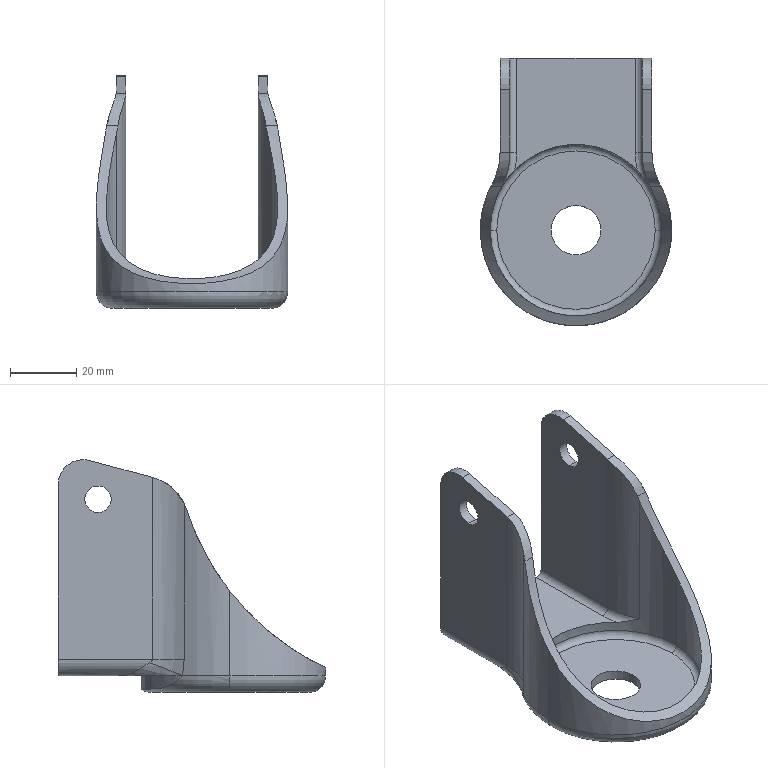Part | SolidWorks | features Cut 4, Fillet 3, Boss 1, Revolution 1 | 1 solid | 48 faces | box 58 x 81 x 70.5 mm | volume 30390 mm3 | cylinder 25 | plane 11 | torus 6 | spline 6 | commonest cylinder face diameters 8 x4 15 x4 58 x3 4 x2 10 x2 30 x2